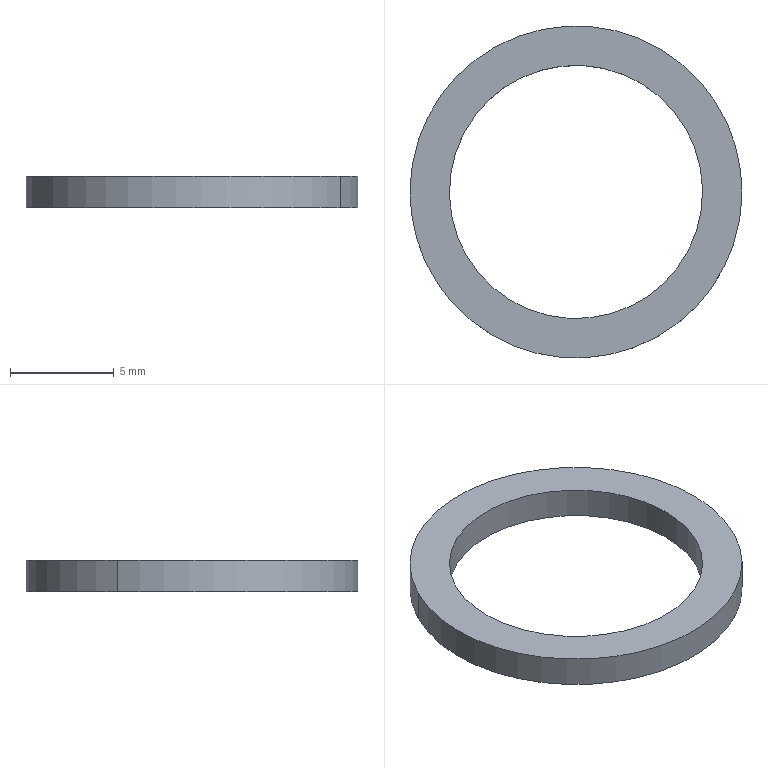Part | SolidWorks | features BaseBody 1 | 1 solid | 6 faces | box 16 x 16 x 1.5 mm | volume 126.245 mm3 | cylinder 4 | plane 2 | commonest cylinder face diameters 12.2 x2 16 x2
STEP:
#1=CARTESIAN_POINT('',(395.544,182.249,-47.));
#2=VERTEX_POINT('',#1);
#3=CARTESIAN_POINT('',(384.656,187.751,-47.));
#4=VERTEX_POINT('',#3);
#5=CARTESIAN_POINT('',(390.1,185.,-47.));
#6=DIRECTION('',(0.,0.,-1.));
#7=DIRECTION('',(-0.8925,0.451,0.));
#8=AXIS2_PLACEMENT_3D('',#5,#6,#7);
#9=CIRCLE('',#8,6.1);
#10=EDGE_CURVE('',#2,#4,#9,.T.);
#11=ORIENTED_EDGE('',*,*,#10,.T.);
#12=CARTESIAN_POINT('',(384.656,187.751,-45.5));
#13=VERTEX_POINT('',#12);
#14=CARTESIAN_POINT('',(384.656,187.751,-47.));
#15=DIRECTION('',(0.,0.,1.));
#16=VECTOR('',#15,1000.);
#17=LINE('',#14,#16);
#18=EDGE_CURVE('',#4,#13,#17,.T.);
#19=ORIENTED_EDGE('',*,*,#18,.T.);
#20=CARTESIAN_POINT('',(395.544,182.249,-45.5));
#21=VERTEX_POINT('',#20);
#22=CARTESIAN_POINT('',(390.1,185.,-45.5));
#23=DIRECTION('',(0.,0.,-1.));
#24=DIRECTION('',(-0.8925,0.451,0.));
#25=AXIS2_PLACEMENT_3D('',#22,#23,#24);
#26=CIRCLE('',#25,6.1);
#27=EDGE_CURVE('',#21,#13,#26,.T.);
#28=ORIENTED_EDGE('',*,*,#27,.F.);
#29=CARTESIAN_POINT('',(395.544,182.249,-47.));
#30=DIRECTION('',(0.,0.,1.));
#31=VECTOR('',#30,1000.);
#32=LINE('',#29,#31);
#33=EDGE_CURVE('',#2,#21,#32,.T.);
#34=ORIENTED_EDGE('',*,*,#33,.F.);
#35=EDGE_LOOP('',(#11,#19,#28,#34));
#36=FACE_OUTER_BOUND('',#35,.T.);
#37=CARTESIAN_POINT('',(390.1,185.,-47.));
#38=DIRECTION('',(0.,0.,1.));
#39=DIRECTION('',(0.8925,-0.451,0.));
#40=AXIS2_PLACEMENT_3D('',#37,#38,#39);
#41=CYLINDRICAL_SURFACE('',#40,6.1);
#42=ADVANCED_FACE('',(#36),#41,.F.);
#43=CARTESIAN_POINT('',(382.96,188.608,-47.));
#44=VERTEX_POINT('',#43);
#45=CARTESIAN_POINT('',(397.24,181.392,-47.));
#46=VERTEX_POINT('',#45);
#47=CARTESIAN_POINT('',(390.1,185.,-47.));
#48=DIRECTION('',(0.,0.,-1.));
#49=DIRECTION('',(-0.8925,0.451,0.));
#50=AXIS2_PLACEMENT_3D('',#47,#48,#49);
#51=CIRCLE('',#50,8.);
#52=EDGE_CURVE('',#44,#46,#51,.T.);
#53=ORIENTED_EDGE('',*,*,#52,.F.);
#54=CARTESIAN_POINT('',(382.96,188.608,-45.5));
#55=VERTEX_POINT('',#54);
#56=CARTESIAN_POINT('',(382.96,188.608,-47.));
#57=DIRECTION('',(0.,0.,1.));
#58=VECTOR('',#57,1000.);
#59=LINE('',#56,#58);
#60=EDGE_CURVE('',#44,#55,#59,.T.);
#61=ORIENTED_EDGE('',*,*,#60,.T.);
#62=CARTESIAN_POINT('',(397.24,181.392,-45.5));
#63=VERTEX_POINT('',#62);
#64=CARTESIAN_POINT('',(390.1,185.,-45.5));
#65=DIRECTION('',(0.,0.,-1.));
#66=DIRECTION('',(-0.8925,0.451,0.));
#67=AXIS2_PLACEMENT_3D('',#64,#65,#66);
#68=CIRCLE('',#67,8.);
#69=EDGE_CURVE('',#55,#63,#68,.T.);
#70=ORIENTED_EDGE('',*,*,#69,.T.);
#71=CARTESIAN_POINT('',(397.24,181.392,-47.));
#72=DIRECTION('',(0.,0.,1.));
#73=VECTOR('',#72,1000.);
#74=LINE('',#71,#73);
#75=EDGE_CURVE('',#46,#63,#74,.T.);
#76=ORIENTED_EDGE('',*,*,#75,.F.);
#77=EDGE_LOOP('',(#53,#61,#70,#76));
#78=FACE_OUTER_BOUND('',#77,.T.);
#79=CARTESIAN_POINT('',(390.1,185.,-47.));
#80=DIRECTION('',(0.,0.,1.));
#81=DIRECTION('',(0.8925,-0.451,0.));
#82=AXIS2_PLACEMENT_3D('',#79,#80,#81);
#83=CYLINDRICAL_SURFACE('',#82,8.);
#84=ADVANCED_FACE('',(#78),#83,.T.);
#85=CARTESIAN_POINT('',(390.1,185.,-47.));
#86=DIRECTION('',(0.,0.,-1.));
#87=DIRECTION('',(-0.8925,0.451,0.));
#88=AXIS2_PLACEMENT_3D('',#85,#86,#87);
#89=CIRCLE('',#88,8.);
#90=EDGE_CURVE('',#46,#44,#89,.T.);
#91=ORIENTED_EDGE('',*,*,#90,.T.);
#92=ORIENTED_EDGE('',*,*,#52,.T.);
#93=EDGE_LOOP('',(#91,#92));
#94=FACE_OUTER_BOUND('',#93,.T.);
#95=ORIENTED_EDGE('',*,*,#10,.F.);
#96=CARTESIAN_POINT('',(390.1,185.,-47.));
#97=DIRECTION('',(0.,0.,-1.));
#98=DIRECTION('',(-0.8925,0.451,0.));
#99=AXIS2_PLACEMENT_3D('',#96,#97,#98);
#100=CIRCLE('',#99,6.1);
#101=EDGE_CURVE('',#4,#2,#100,.T.);
#102=ORIENTED_EDGE('',*,*,#101,.F.);
#103=EDGE_LOOP('',(#95,#102));
#104=FACE_BOUND('',#103,.T.);
#105=CARTESIAN_POINT('',(390.1,185.,-47.));
#106=DIRECTION('',(0.,0.,-1.));
#107=DIRECTION('',(-0.8925,0.451,0.));
#108=AXIS2_PLACEMENT_3D('',#105,#106,#107);
#109=PLANE('',#108);
#110=ADVANCED_FACE('',(#94,#104),#109,.T.);
#111=CARTESIAN_POINT('',(390.1,185.,-45.5));
#112=DIRECTION('',(0.,0.,-1.));
#113=DIRECTION('',(-0.8925,0.451,0.));
#114=AXIS2_PLACEMENT_3D('',#111,#112,#113);
#115=CIRCLE('',#114,8.);
#116=EDGE_CURVE('',#63,#55,#115,.T.);
#117=ORIENTED_EDGE('',*,*,#116,.F.);
#118=ORIENTED_EDGE('',*,*,#69,.F.);
#119=EDGE_LOOP('',(#117,#118));
#120=FACE_OUTER_BOUND('',#119,.T.);
#121=ORIENTED_EDGE('',*,*,#27,.T.);
#122=CARTESIAN_POINT('',(390.1,185.,-45.5));
#123=DIRECTION('',(0.,0.,-1.));
#124=DIRECTION('',(-0.8925,0.451,0.));
#125=AXIS2_PLACEMENT_3D('',#122,#123,#124);
#126=CIRCLE('',#125,6.1);
#127=EDGE_CURVE('',#13,#21,#126,.T.);
#128=ORIENTED_EDGE('',*,*,#127,.T.);
#129=EDGE_LOOP('',(#121,#128));
#130=FACE_BOUND('',#129,.T.);
#131=CARTESIAN_POINT('',(390.1,185.,-45.5));
#132=DIRECTION('',(0.,0.,-1.));
#133=DIRECTION('',(-0.8925,0.451,0.));
#134=AXIS2_PLACEMENT_3D('',#131,#132,#133);
#135=PLANE('',#134);
#136=ADVANCED_FACE('',(#120,#130),#135,.F.);
#137=ORIENTED_EDGE('',*,*,#60,.F.);
#138=ORIENTED_EDGE('',*,*,#90,.F.);
#139=ORIENTED_EDGE('',*,*,#75,.T.);
#140=ORIENTED_EDGE('',*,*,#116,.T.);
#141=EDGE_LOOP('',(#137,#138,#139,#140));
#142=FACE_OUTER_BOUND('',#141,.T.);
#143=CARTESIAN_POINT('',(390.1,185.,-47.));
#144=DIRECTION('',(0.,0.,1.));
#145=DIRECTION('',(0.8925,-0.451,0.));
#146=AXIS2_PLACEMENT_3D('',#143,#144,#145);
#147=CYLINDRICAL_SURFACE('',#146,8.);
#148=ADVANCED_FACE('',(#142),#147,.T.);
#149=ORIENTED_EDGE('',*,*,#18,.F.);
#150=ORIENTED_EDGE('',*,*,#101,.T.);
#151=ORIENTED_EDGE('',*,*,#33,.T.);
#152=ORIENTED_EDGE('',*,*,#127,.F.);
#153=EDGE_LOOP('',(#149,#150,#151,#152));
#154=FACE_OUTER_BOUND('',#153,.T.);
#155=CARTESIAN_POINT('',(390.1,185.,-47.));
#156=DIRECTION('',(0.,0.,1.));
#157=DIRECTION('',(0.8925,-0.451,0.));
#158=AXIS2_PLACEMENT_3D('',#155,#156,#157);
#159=CYLINDRICAL_SURFACE('',#158,6.1);
#160=ADVANCED_FACE('',(#154),#159,.F.);
#161=CLOSED_SHELL('',(#42,#84,#110,#136,#148,#160));
#162=MANIFOLD_SOLID_BREP('',#161);
#163=CARTESIAN_POINT('',(0.,0.,0.));
#164=DIRECTION('',(0.,0.,1.));
#165=DIRECTION('',(1.,0.,0.));
#166=AXIS2_PLACEMENT_3D('',#163,#164,#165);
#167=(LENGTH_UNIT()NAMED_UNIT(*)SI_UNIT(.MILLI.,.METRE.));
#168=UNCERTAINTY_MEASURE_WITH_UNIT(LENGTH_MEASURE(0.00001),#167,'','');
#169=(NAMED_UNIT(*)PLANE_ANGLE_UNIT()SI_UNIT($,.RADIAN.));
#170=(NAMED_UNIT(*)SI_UNIT($,.STERADIAN.)SOLID_ANGLE_UNIT());
#171=(GEOMETRIC_REPRESENTATION_CONTEXT(3)GLOBAL_UNCERTAINTY_ASSIGNED_CONTEXT((#168))GLOBAL_UNIT_ASSIGNED_CONTEXT((#167,#169,#170))REPRESENTATION_CONTEXT('',''));
#172=ADVANCED_BREP_SHAPE_REPRESENTATION('',(#162,#166),#171);